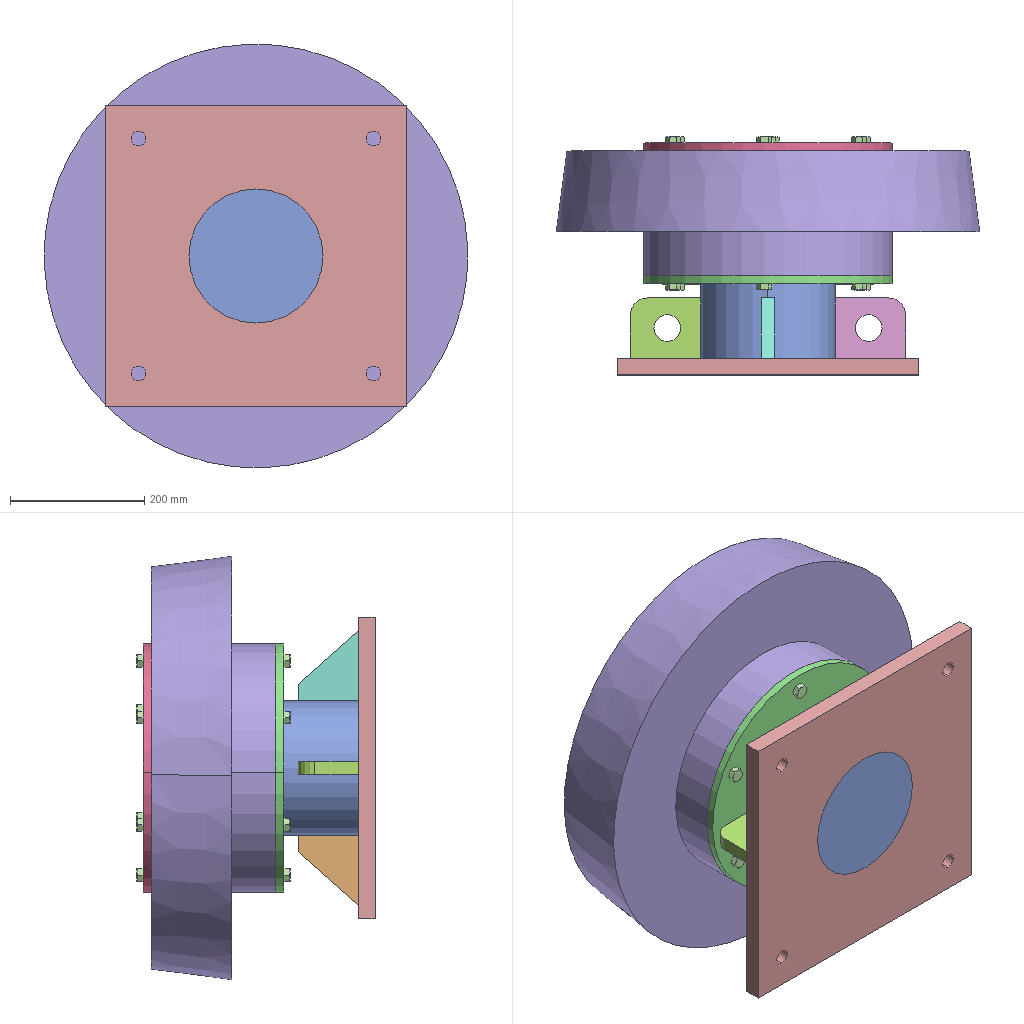Assembly | SolidWorks | 11 different items | 50 placed | box 631 x 355 x 631 mm
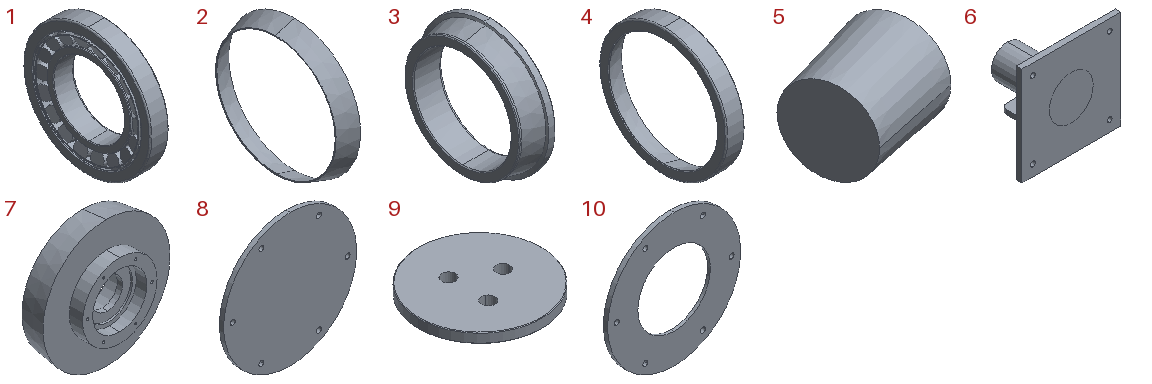Parts list (item | name | quantity | parent item | size | volume | features):
1 | (subassembly) | x2 | - | 49.167 x 270 x 270 mm | 1287468 mm3 | -
2 | - | x2 | in 1 | 34.434 x 242.32 x 242.32 mm | 26377 mm3 | features BaseBody 1
3 | - | x2 | in 1 | 45 x 200.13 x 200.13 mm | 409638 mm3 | features BaseBody 1
4 | - | x2 | in 1 | 38 x 270 x 270 mm | 453986 mm3 | features BaseBody 1
5 | - | x36 | in 1 | 37.94 x 36.648 x 30.927 mm | 22081 mm3 | features BaseBody 1
6 | - | x1 | - | 450 x 291 x 450 mm | 11988612 mm3 | features ICE 7, Fillet 2, 3DProfileFeature 1, Chamfer 1, CirPattern 1, Extrusion 1, HoleWzd 1
7 | - | x1 | - | 631.597 x 186 x 631.597 mm | 33435702 mm3 | features 3DProfileFeature 2, CirPattern 2, HoleWzd 2, Revolution 1
8 | - | x1 | - | 370 x 16 x 370 mm | 1084232 mm3 | features ICE 3, CirPattern 1, Extrusion 1
9 | - | x1 | - | 200 x 200 x 16 mm | 483782 mm3 | features Chamfer 1, CirPattern 1, Extrusion 1, ICE 1
10 | - | x1 | - | 370 x 16 x 370 mm | 827853 mm3 | features ICE 3, CirPattern 1, Extrusion 1
11 | hex bolt_ai | x1 | - | - | - | -
Mates (type | each side: item.copy, entity, surface, feature):
Concentric | 7.1 face cylinder Revolve1 | 3.1 face cylinder 30230_ir
Coincident | 7.1 face plane Revolve1 | 4.1 face plane 30230_or
Concentric | 7.1 face cylinder Revolve1 | 3.2 face cylinder 30230_ir
Coincident | 7.1 face plane Revolve1 | 4.2 face plane 30230_or
Concentric | 7.1 face cylinder Revolve1 | 10.1 face cylinder Boss-Extrude2
Concentric | 7.1 face cylinder CirPattern2 | 10.1 face cylinder CirPattern1
Coincident | 7.1 face plane Revolve1 | 10.1 face plane Boss-Extrude1
Concentric | 6.1 face cylinder Boss-Extrude4 | 3.1 face cylinder 30230_ir
Coincident | 6.1 face plane Boss-Extrude3 | 3.2 face plane 30230_ir
Concentric | 6.1 edge | 9.1 face cylinder Boss-Extrude1
Concentric | 6.1 face cylinder 3/4-10 Tapped Hole1 | 9.1 face cylinder Cut-Extrude1
Coincident | 6.1 face plane Boss-Extrude4 | 9.1 face plane Boss-Extrude1
Concentric | 7.1 face cylinder Revolve1 | 8.1 face cylinder Boss-Extrude2
Concentric | 7.1 face cylinder 1/2-13 Tapped Hole1 | 8.1 face cylinder CirPattern2
Coincident | 7.1 face plane Revolve1 | 8.1 face plane Boss-Extrude1